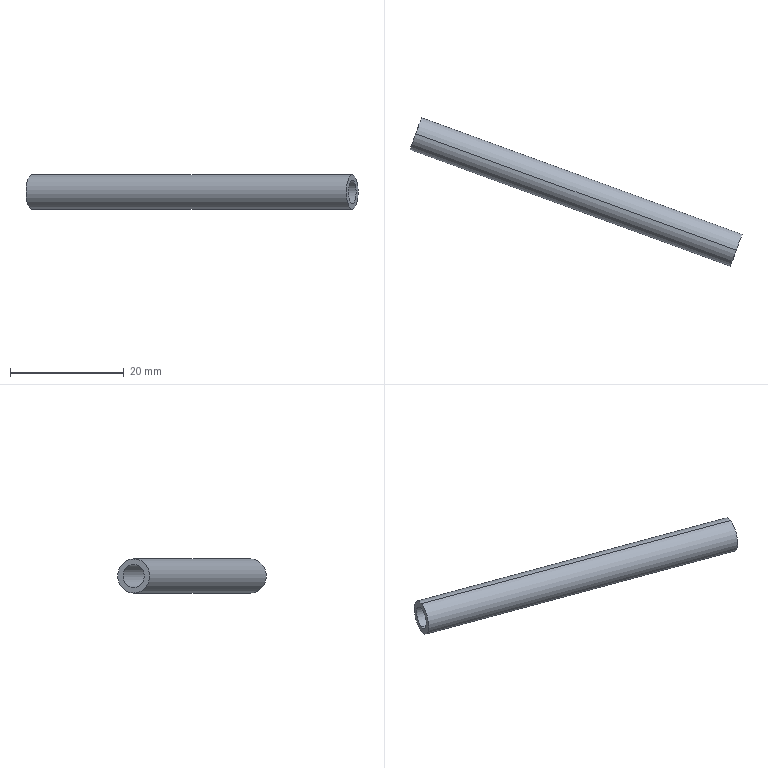Part | SolidWorks | features BaseBody 1 | 1 solid | 6 faces | box 58.434 x 26.159 x 6 mm | volume 942.478 mm3 | cylinder 4 | plane 2 | commonest cylinder face diameters 4 x2 6 x2
STEP:
#1=CARTESIAN_POINT('',(-185.494,83.749,-245.5));
#2=VERTEX_POINT('',#1);
#3=CARTESIAN_POINT('',(-185.494,83.749,-249.5));
#4=VERTEX_POINT('',#3);
#5=CARTESIAN_POINT('',(-185.494,83.749,-247.5));
#6=DIRECTION('',(0.9397,-0.342,0.));
#7=DIRECTION('',(-0.342,-0.9397,0.));
#8=AXIS2_PLACEMENT_3D('',#5,#6,#7);
#9=CIRCLE('',#8,2.);
#10=EDGE_CURVE('',#2,#4,#9,.T.);
#11=ORIENTED_EDGE('',*,*,#10,.F.);
#12=CARTESIAN_POINT('',(-129.113,63.228,-245.5));
#13=VERTEX_POINT('',#12);
#14=CARTESIAN_POINT('',(-129.113,63.228,-245.5));
#15=DIRECTION('',(0.9397,-0.342,0.));
#16=VECTOR('',#15,1000.);
#17=LINE('',#14,#16);
#18=EDGE_CURVE('',#2,#13,#17,.T.);
#19=ORIENTED_EDGE('',*,*,#18,.T.);
#20=CARTESIAN_POINT('',(-129.113,63.228,-249.5));
#21=VERTEX_POINT('',#20);
#22=CARTESIAN_POINT('',(-129.113,63.228,-247.5));
#23=DIRECTION('',(0.9397,-0.342,0.));
#24=DIRECTION('',(0.,0.,-1.));
#25=AXIS2_PLACEMENT_3D('',#22,#23,#24);
#26=CIRCLE('',#25,2.);
#27=EDGE_CURVE('',#13,#21,#26,.T.);
#28=ORIENTED_EDGE('',*,*,#27,.T.);
#29=CARTESIAN_POINT('',(-129.113,63.228,-249.5));
#30=DIRECTION('',(0.9397,-0.342,0.));
#31=VECTOR('',#30,1000.);
#32=LINE('',#29,#31);
#33=EDGE_CURVE('',#4,#21,#32,.T.);
#34=ORIENTED_EDGE('',*,*,#33,.F.);
#35=EDGE_LOOP('',(#11,#19,#28,#34));
#36=FACE_OUTER_BOUND('',#35,.T.);
#37=CARTESIAN_POINT('',(-129.113,63.228,-247.5));
#38=DIRECTION('',(0.9397,-0.342,0.));
#39=DIRECTION('',(0.,0.,-1.));
#40=AXIS2_PLACEMENT_3D('',#37,#38,#39);
#41=CYLINDRICAL_SURFACE('',#40,2.);
#42=ADVANCED_FACE('',(#36),#41,.F.);
#43=CARTESIAN_POINT('',(-185.494,83.749,-250.5));
#44=VERTEX_POINT('',#43);
#45=CARTESIAN_POINT('',(-185.494,83.749,-244.5));
#46=VERTEX_POINT('',#45);
#47=CARTESIAN_POINT('',(-185.494,83.749,-247.5));
#48=DIRECTION('',(0.9397,-0.342,0.));
#49=DIRECTION('',(-0.342,-0.9397,0.));
#50=AXIS2_PLACEMENT_3D('',#47,#48,#49);
#51=CIRCLE('',#50,3.);
#52=EDGE_CURVE('',#44,#46,#51,.T.);
#53=ORIENTED_EDGE('',*,*,#52,.T.);
#54=CARTESIAN_POINT('',(-129.113,63.228,-244.5));
#55=VERTEX_POINT('',#54);
#56=CARTESIAN_POINT('',(-129.113,63.228,-244.5));
#57=DIRECTION('',(0.9397,-0.342,0.));
#58=VECTOR('',#57,1000.);
#59=LINE('',#56,#58);
#60=EDGE_CURVE('',#46,#55,#59,.T.);
#61=ORIENTED_EDGE('',*,*,#60,.T.);
#62=CARTESIAN_POINT('',(-129.113,63.228,-250.5));
#63=VERTEX_POINT('',#62);
#64=CARTESIAN_POINT('',(-129.113,63.228,-247.5));
#65=DIRECTION('',(0.9397,-0.342,0.));
#66=DIRECTION('',(0.,0.,-1.));
#67=AXIS2_PLACEMENT_3D('',#64,#65,#66);
#68=CIRCLE('',#67,3.);
#69=EDGE_CURVE('',#63,#55,#68,.T.);
#70=ORIENTED_EDGE('',*,*,#69,.F.);
#71=CARTESIAN_POINT('',(-129.113,63.228,-250.5));
#72=DIRECTION('',(0.9397,-0.342,0.));
#73=VECTOR('',#72,1000.);
#74=LINE('',#71,#73);
#75=EDGE_CURVE('',#44,#63,#74,.T.);
#76=ORIENTED_EDGE('',*,*,#75,.F.);
#77=EDGE_LOOP('',(#53,#61,#70,#76));
#78=FACE_OUTER_BOUND('',#77,.T.);
#79=CARTESIAN_POINT('',(-129.113,63.228,-247.5));
#80=DIRECTION('',(0.9397,-0.342,0.));
#81=DIRECTION('',(0.,0.,-1.));
#82=AXIS2_PLACEMENT_3D('',#79,#80,#81);
#83=CYLINDRICAL_SURFACE('',#82,3.);
#84=ADVANCED_FACE('',(#78),#83,.T.);
#85=ORIENTED_EDGE('',*,*,#60,.F.);
#86=CARTESIAN_POINT('',(-185.494,83.749,-247.5));
#87=DIRECTION('',(0.9397,-0.342,0.));
#88=DIRECTION('',(-0.342,-0.9397,0.));
#89=AXIS2_PLACEMENT_3D('',#86,#87,#88);
#90=CIRCLE('',#89,3.);
#91=EDGE_CURVE('',#46,#44,#90,.T.);
#92=ORIENTED_EDGE('',*,*,#91,.T.);
#93=ORIENTED_EDGE('',*,*,#75,.T.);
#94=CARTESIAN_POINT('',(-129.113,63.228,-247.5));
#95=DIRECTION('',(0.9397,-0.342,0.));
#96=DIRECTION('',(0.,0.,-1.));
#97=AXIS2_PLACEMENT_3D('',#94,#95,#96);
#98=CIRCLE('',#97,3.);
#99=EDGE_CURVE('',#55,#63,#98,.T.);
#100=ORIENTED_EDGE('',*,*,#99,.F.);
#101=EDGE_LOOP('',(#85,#92,#93,#100));
#102=FACE_OUTER_BOUND('',#101,.T.);
#103=CARTESIAN_POINT('',(-129.113,63.228,-247.5));
#104=DIRECTION('',(0.9397,-0.342,0.));
#105=DIRECTION('',(0.,0.,-1.));
#106=AXIS2_PLACEMENT_3D('',#103,#104,#105);
#107=CYLINDRICAL_SURFACE('',#106,3.);
#108=ADVANCED_FACE('',(#102),#107,.T.);
#109=CARTESIAN_POINT('',(-185.494,83.749,-247.5));
#110=DIRECTION('',(0.9397,-0.342,0.));
#111=DIRECTION('',(-0.342,-0.9397,0.));
#112=AXIS2_PLACEMENT_3D('',#109,#110,#111);
#113=CIRCLE('',#112,2.);
#114=EDGE_CURVE('',#4,#2,#113,.T.);
#115=ORIENTED_EDGE('',*,*,#114,.T.);
#116=ORIENTED_EDGE('',*,*,#10,.T.);
#117=EDGE_LOOP('',(#115,#116));
#118=FACE_BOUND('',#117,.T.);
#119=ORIENTED_EDGE('',*,*,#52,.F.);
#120=ORIENTED_EDGE('',*,*,#91,.F.);
#121=EDGE_LOOP('',(#119,#120));
#122=FACE_OUTER_BOUND('',#121,.T.);
#123=CARTESIAN_POINT('',(-184.468,86.568,-247.5));
#124=DIRECTION('',(-0.9397,0.342,0.));
#125=DIRECTION('',(0.,0.,1.));
#126=AXIS2_PLACEMENT_3D('',#123,#124,#125);
#127=PLANE('',#126);
#128=ADVANCED_FACE('',(#118,#122),#127,.T.);
#129=ORIENTED_EDGE('',*,*,#18,.F.);
#130=ORIENTED_EDGE('',*,*,#114,.F.);
#131=ORIENTED_EDGE('',*,*,#33,.T.);
#132=CARTESIAN_POINT('',(-129.113,63.228,-247.5));
#133=DIRECTION('',(0.9397,-0.342,0.));
#134=DIRECTION('',(0.,0.,-1.));
#135=AXIS2_PLACEMENT_3D('',#132,#133,#134);
#136=CIRCLE('',#135,2.);
#137=EDGE_CURVE('',#21,#13,#136,.T.);
#138=ORIENTED_EDGE('',*,*,#137,.T.);
#139=EDGE_LOOP('',(#129,#130,#131,#138));
#140=FACE_OUTER_BOUND('',#139,.T.);
#141=CARTESIAN_POINT('',(-129.113,63.228,-247.5));
#142=DIRECTION('',(0.9397,-0.342,0.));
#143=DIRECTION('',(0.,0.,-1.));
#144=AXIS2_PLACEMENT_3D('',#141,#142,#143);
#145=CYLINDRICAL_SURFACE('',#144,2.);
#146=ADVANCED_FACE('',(#140),#145,.F.);
#147=ORIENTED_EDGE('',*,*,#69,.T.);
#148=ORIENTED_EDGE('',*,*,#99,.T.);
#149=EDGE_LOOP('',(#147,#148));
#150=FACE_OUTER_BOUND('',#149,.T.);
#151=ORIENTED_EDGE('',*,*,#137,.F.);
#152=ORIENTED_EDGE('',*,*,#27,.F.);
#153=EDGE_LOOP('',(#151,#152));
#154=FACE_BOUND('',#153,.T.);
#155=CARTESIAN_POINT('',(-128.429,65.107,-247.5));
#156=DIRECTION('',(0.9397,-0.342,0.));
#157=DIRECTION('',(0.,0.,-1.));
#158=AXIS2_PLACEMENT_3D('',#155,#156,#157);
#159=PLANE('',#158);
#160=ADVANCED_FACE('',(#150,#154),#159,.T.);
#161=CLOSED_SHELL('',(#42,#84,#108,#128,#146,#160));
#162=MANIFOLD_SOLID_BREP('',#161);
#163=CARTESIAN_POINT('',(0.,0.,0.));
#164=DIRECTION('',(0.,0.,1.));
#165=DIRECTION('',(1.,0.,0.));
#166=AXIS2_PLACEMENT_3D('',#163,#164,#165);
#167=(LENGTH_UNIT()NAMED_UNIT(*)SI_UNIT(.MILLI.,.METRE.));
#168=UNCERTAINTY_MEASURE_WITH_UNIT(LENGTH_MEASURE(0.00001),#167,'','');
#169=(NAMED_UNIT(*)PLANE_ANGLE_UNIT()SI_UNIT($,.RADIAN.));
#170=(NAMED_UNIT(*)SI_UNIT($,.STERADIAN.)SOLID_ANGLE_UNIT());
#171=(GEOMETRIC_REPRESENTATION_CONTEXT(3)GLOBAL_UNCERTAINTY_ASSIGNED_CONTEXT((#168))GLOBAL_UNIT_ASSIGNED_CONTEXT((#167,#169,#170))REPRESENTATION_CONTEXT('',''));
#172=ADVANCED_BREP_SHAPE_REPRESENTATION('',(#162,#166),#171);